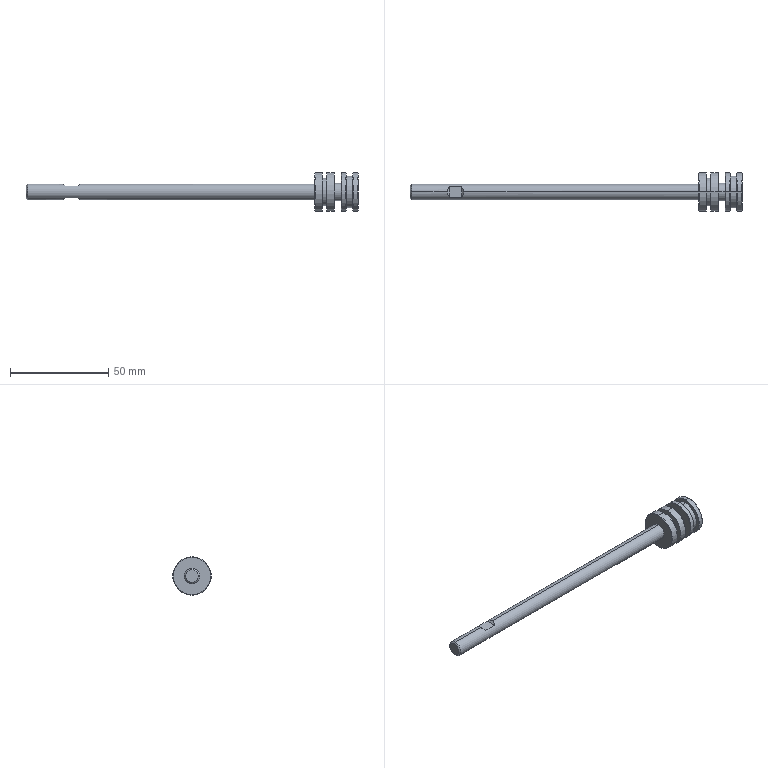Part | STEP file | Copy 2^MA20-80-S-U | 1 solid | 45 faces | box 169 x 19.5 x 19.5 mm | volume 12396 mm3 | cylinder 16 | plane 15 | cone 14 | commonest cylinder face diameters 19.5 x8 8 x2 8.9 x2 14 x2 16 x2
STEP:
#1=CARTESIAN_POINT('',(-55.233,0.,-4.));
#2=VERTEX_POINT('',#1);
#3=CARTESIAN_POINT('',(-55.233,0.,4.));
#4=VERTEX_POINT('',#3);
#5=CARTESIAN_POINT('',(-55.233,0.,0.));
#6=DIRECTION('',(1.,0.,0.));
#7=DIRECTION('',(0.,0.,-1.));
#8=AXIS2_PLACEMENT_3D('',#5,#6,#7);
#9=CIRCLE('',#8,4.);
#10=EDGE_CURVE('',#2,#4,#9,.T.);
#11=ORIENTED_EDGE('',*,*,#10,.T.);
#12=CARTESIAN_POINT('',(-37.,0.,4.));
#13=VERTEX_POINT('',#12);
#14=CARTESIAN_POINT('',(17.884,0.,4.));
#15=DIRECTION('',(1.,0.,0.));
#16=VECTOR('',#15,1000.);
#17=LINE('',#14,#16);
#18=EDGE_CURVE('',#4,#13,#17,.T.);
#19=ORIENTED_EDGE('',*,*,#18,.T.);
#20=CARTESIAN_POINT('',(-36.,2.646,3.));
#21=VERTEX_POINT('',#20);
#22=CARTESIAN_POINT('',(-37.,0.,4.));
#23=CARTESIAN_POINT('',(-37.,0.9852,4.));
#24=CARTESIAN_POINT('',(-36.652,1.907,3.652));
#25=CARTESIAN_POINT('',(-36.,2.646,3.));
#26=(BOUNDED_CURVE()B_SPLINE_CURVE(3,(#22,#23,#24,#25),.UNSPECIFIED.,.F.,.F.)B_SPLINE_CURVE_WITH_KNOTS((4,4),(3.142,3.864),.UNSPECIFIED.)CURVE()GEOMETRIC_REPRESENTATION_ITEM()RATIONAL_B_SPLINE_CURVE((1.,0.9569,0.9569,1.))REPRESENTATION_ITEM(''));
#27=EDGE_CURVE('',#13,#21,#26,.T.);
#28=ORIENTED_EDGE('',*,*,#27,.T.);
#29=CARTESIAN_POINT('',(-29.6,2.646,3.));
#30=VERTEX_POINT('',#29);
#31=CARTESIAN_POINT('',(17.884,2.646,3.));
#32=DIRECTION('',(1.,0.,0.));
#33=VECTOR('',#32,1000.);
#34=LINE('',#31,#33);
#35=EDGE_CURVE('',#21,#30,#34,.T.);
#36=ORIENTED_EDGE('',*,*,#35,.T.);
#37=CARTESIAN_POINT('',(-28.6,0.,4.));
#38=VERTEX_POINT('',#37);
#39=CARTESIAN_POINT('',(-29.6,2.646,3.));
#40=CARTESIAN_POINT('',(-28.948,1.907,3.652));
#41=CARTESIAN_POINT('',(-28.6,0.9852,4.));
#42=CARTESIAN_POINT('',(-28.6,0.,4.));
#43=(BOUNDED_CURVE()B_SPLINE_CURVE(3,(#39,#40,#41,#42),.UNSPECIFIED.,.F.,.F.)B_SPLINE_CURVE_WITH_KNOTS((4,4),(5.56,6.283),.UNSPECIFIED.)CURVE()GEOMETRIC_REPRESENTATION_ITEM()RATIONAL_B_SPLINE_CURVE((1.,0.9569,0.9569,1.))REPRESENTATION_ITEM(''));
#44=EDGE_CURVE('',#30,#38,#43,.T.);
#45=ORIENTED_EDGE('',*,*,#44,.T.);
#46=CARTESIAN_POINT('',(91.,0.,4.));
#47=VERTEX_POINT('',#46);
#48=CARTESIAN_POINT('',(17.884,0.,4.));
#49=DIRECTION('',(1.,0.,0.));
#50=VECTOR('',#49,1000.);
#51=LINE('',#48,#50);
#52=EDGE_CURVE('',#38,#47,#51,.T.);
#53=ORIENTED_EDGE('',*,*,#52,.T.);
#54=CARTESIAN_POINT('',(91.,0.,-4.));
#55=VERTEX_POINT('',#54);
#56=CARTESIAN_POINT('',(91.,0.,0.));
#57=DIRECTION('',(-1.,0.,0.));
#58=DIRECTION('',(0.,0.,-1.));
#59=AXIS2_PLACEMENT_3D('',#56,#57,#58);
#60=CIRCLE('',#59,4.);
#61=EDGE_CURVE('',#47,#55,#60,.T.);
#62=ORIENTED_EDGE('',*,*,#61,.T.);
#63=CARTESIAN_POINT('',(-28.6,0.,-4.));
#64=VERTEX_POINT('',#63);
#65=CARTESIAN_POINT('',(17.884,0.,-4.));
#66=DIRECTION('',(1.,0.,0.));
#67=VECTOR('',#66,1000.);
#68=LINE('',#65,#67);
#69=EDGE_CURVE('',#64,#55,#68,.T.);
#70=ORIENTED_EDGE('',*,*,#69,.F.);
#71=CARTESIAN_POINT('',(-29.6,2.646,-3.));
#72=VERTEX_POINT('',#71);
#73=CARTESIAN_POINT('',(-28.6,0.,-4.));
#74=CARTESIAN_POINT('',(-28.6,0.9852,-4.));
#75=CARTESIAN_POINT('',(-28.948,1.907,-3.652));
#76=CARTESIAN_POINT('',(-29.6,2.646,-3.));
#77=(BOUNDED_CURVE()B_SPLINE_CURVE(3,(#73,#74,#75,#76),.UNSPECIFIED.,.F.,.F.)B_SPLINE_CURVE_WITH_KNOTS((4,4),(0.,0.7227),.UNSPECIFIED.)CURVE()GEOMETRIC_REPRESENTATION_ITEM()RATIONAL_B_SPLINE_CURVE((1.,0.9569,0.9569,1.))REPRESENTATION_ITEM(''));
#78=EDGE_CURVE('',#64,#72,#77,.T.);
#79=ORIENTED_EDGE('',*,*,#78,.T.);
#80=CARTESIAN_POINT('',(-36.,2.646,-3.));
#81=VERTEX_POINT('',#80);
#82=CARTESIAN_POINT('',(17.884,2.646,-3.));
#83=DIRECTION('',(-1.,0.,0.));
#84=VECTOR('',#83,1000.);
#85=LINE('',#82,#84);
#86=EDGE_CURVE('',#72,#81,#85,.T.);
#87=ORIENTED_EDGE('',*,*,#86,.T.);
#88=CARTESIAN_POINT('',(-37.,0.,-4.));
#89=VERTEX_POINT('',#88);
#90=CARTESIAN_POINT('',(-36.,2.646,-3.));
#91=CARTESIAN_POINT('',(-36.652,1.907,-3.652));
#92=CARTESIAN_POINT('',(-37.,0.9852,-4.));
#93=CARTESIAN_POINT('',(-37.,0.,-4.));
#94=(BOUNDED_CURVE()B_SPLINE_CURVE(3,(#90,#91,#92,#93),.UNSPECIFIED.,.F.,.F.)B_SPLINE_CURVE_WITH_KNOTS((4,4),(2.419,3.142),.UNSPECIFIED.)CURVE()GEOMETRIC_REPRESENTATION_ITEM()RATIONAL_B_SPLINE_CURVE((1.,0.9569,0.9569,1.))REPRESENTATION_ITEM(''));
#95=EDGE_CURVE('',#81,#89,#94,.T.);
#96=ORIENTED_EDGE('',*,*,#95,.T.);
#97=CARTESIAN_POINT('',(17.884,0.,-4.));
#98=DIRECTION('',(1.,0.,0.));
#99=VECTOR('',#98,1000.);
#100=LINE('',#97,#99);
#101=EDGE_CURVE('',#2,#89,#100,.T.);
#102=ORIENTED_EDGE('',*,*,#101,.F.);
#103=EDGE_LOOP('',(#11,#19,#28,#36,#45,#53,#62,#70,#79,#87,#96,#102));
#104=FACE_OUTER_BOUND('',#103,.T.);
#105=CARTESIAN_POINT('',(17.884,0.,0.));
#106=DIRECTION('',(1.,0.,0.));
#107=DIRECTION('',(0.,0.,-1.));
#108=AXIS2_PLACEMENT_3D('',#105,#106,#107);
#109=CYLINDRICAL_SURFACE('',#108,4.);
#110=ADVANCED_FACE('',(#104),#109,.T.);
#111=CARTESIAN_POINT('',(-56.,0.,-3.233));
#112=VERTEX_POINT('',#111);
#113=CARTESIAN_POINT('',(-56.,0.,3.233));
#114=VERTEX_POINT('',#113);
#115=CARTESIAN_POINT('',(-56.,0.,0.));
#116=DIRECTION('',(1.,0.,0.));
#117=DIRECTION('',(0.,0.,-1.));
#118=AXIS2_PLACEMENT_3D('',#115,#116,#117);
#119=CIRCLE('',#118,3.233);
#120=EDGE_CURVE('',#112,#114,#119,.T.);
#121=ORIENTED_EDGE('',*,*,#120,.T.);
#122=CARTESIAN_POINT('',(-55.233,0.,4.));
#123=DIRECTION('',(0.7071,0.,0.7071));
#124=VECTOR('',#123,1000.);
#125=LINE('',#122,#124);
#126=EDGE_CURVE('',#114,#4,#125,.T.);
#127=ORIENTED_EDGE('',*,*,#126,.T.);
#128=ORIENTED_EDGE('',*,*,#10,.F.);
#129=CARTESIAN_POINT('',(-55.233,0.,-4.));
#130=DIRECTION('',(0.7071,0.,-0.7071));
#131=VECTOR('',#130,1000.);
#132=LINE('',#129,#131);
#133=EDGE_CURVE('',#112,#2,#132,.T.);
#134=ORIENTED_EDGE('',*,*,#133,.F.);
#135=EDGE_LOOP('',(#121,#127,#128,#134));
#136=FACE_OUTER_BOUND('',#135,.T.);
#137=CARTESIAN_POINT('',(-55.233,0.,0.));
#138=DIRECTION('',(1.,0.,0.));
#139=DIRECTION('',(0.,0.,-1.));
#140=AXIS2_PLACEMENT_3D('',#137,#138,#139);
#141=CONICAL_SURFACE('',#140,4.,0.7854);
#142=ADVANCED_FACE('',(#136),#141,.T.);
#143=CARTESIAN_POINT('',(91.,0.,9.55));
#144=VERTEX_POINT('',#143);
#145=CARTESIAN_POINT('',(91.,0.,-9.55));
#146=VERTEX_POINT('',#145);
#147=CARTESIAN_POINT('',(91.,0.,0.));
#148=DIRECTION('',(-1.,0.,0.));
#149=DIRECTION('',(0.,0.,-1.));
#150=AXIS2_PLACEMENT_3D('',#147,#148,#149);
#151=CIRCLE('',#150,9.55);
#152=EDGE_CURVE('',#144,#146,#151,.T.);
#153=ORIENTED_EDGE('',*,*,#152,.F.);
#154=CARTESIAN_POINT('',(91.2,0.,9.75));
#155=VERTEX_POINT('',#154);
#156=CARTESIAN_POINT('',(91.2,0.,9.75));
#157=DIRECTION('',(0.7071,0.,0.7071));
#158=VECTOR('',#157,1000.);
#159=LINE('',#156,#158);
#160=EDGE_CURVE('',#144,#155,#159,.T.);
#161=ORIENTED_EDGE('',*,*,#160,.T.);
#162=CARTESIAN_POINT('',(91.2,0.,-9.75));
#163=VERTEX_POINT('',#162);
#164=CARTESIAN_POINT('',(91.2,0.,0.));
#165=DIRECTION('',(-1.,0.,0.));
#166=DIRECTION('',(0.,1.,0.));
#167=AXIS2_PLACEMENT_3D('',#164,#165,#166);
#168=CIRCLE('',#167,9.75);
#169=EDGE_CURVE('',#155,#163,#168,.T.);
#170=ORIENTED_EDGE('',*,*,#169,.T.);
#171=CARTESIAN_POINT('',(91.2,0.,-9.75));
#172=DIRECTION('',(0.7071,0.,-0.7071));
#173=VECTOR('',#172,1000.);
#174=LINE('',#171,#173);
#175=EDGE_CURVE('',#146,#163,#174,.T.);
#176=ORIENTED_EDGE('',*,*,#175,.F.);
#177=EDGE_LOOP('',(#153,#161,#170,#176));
#178=FACE_OUTER_BOUND('',#177,.T.);
#179=CARTESIAN_POINT('',(91.2,0.,0.));
#180=DIRECTION('',(1.,0.,0.));
#181=DIRECTION('',(0.,0.,-1.));
#182=AXIS2_PLACEMENT_3D('',#179,#180,#181);
#183=CONICAL_SURFACE('',#182,9.75,0.7854);
#184=ADVANCED_FACE('',(#178),#183,.T.);
#185=ORIENTED_EDGE('',*,*,#169,.F.);
#186=CARTESIAN_POINT('',(94.8,0.,9.75));
#187=VERTEX_POINT('',#186);
#188=CARTESIAN_POINT('',(93.,0.,9.75));
#189=DIRECTION('',(1.,0.,0.));
#190=VECTOR('',#189,1000.);
#191=LINE('',#188,#190);
#192=EDGE_CURVE('',#155,#187,#191,.T.);
#193=ORIENTED_EDGE('',*,*,#192,.T.);
#194=CARTESIAN_POINT('',(94.8,0.,-9.75));
#195=VERTEX_POINT('',#194);
#196=CARTESIAN_POINT('',(94.8,0.,0.));
#197=DIRECTION('',(-1.,0.,0.));
#198=DIRECTION('',(0.,0.,-1.));
#199=AXIS2_PLACEMENT_3D('',#196,#197,#198);
#200=CIRCLE('',#199,9.75);
#201=EDGE_CURVE('',#187,#195,#200,.T.);
#202=ORIENTED_EDGE('',*,*,#201,.T.);
#203=CARTESIAN_POINT('',(93.,0.,-9.75));
#204=DIRECTION('',(1.,0.,0.));
#205=VECTOR('',#204,1000.);
#206=LINE('',#203,#205);
#207=EDGE_CURVE('',#163,#195,#206,.T.);
#208=ORIENTED_EDGE('',*,*,#207,.F.);
#209=EDGE_LOOP('',(#185,#193,#202,#208));
#210=FACE_OUTER_BOUND('',#209,.T.);
#211=CARTESIAN_POINT('',(93.,0.,0.));
#212=DIRECTION('',(1.,0.,0.));
#213=DIRECTION('',(0.,0.,-1.));
#214=AXIS2_PLACEMENT_3D('',#211,#212,#213);
#215=CYLINDRICAL_SURFACE('',#214,9.75);
#216=ADVANCED_FACE('',(#210),#215,.T.);
#217=CARTESIAN_POINT('',(94.8,0.,7.));
#218=VERTEX_POINT('',#217);
#219=CARTESIAN_POINT('',(94.8,0.,-7.));
#220=VERTEX_POINT('',#219);
#221=CARTESIAN_POINT('',(94.8,0.,0.));
#222=DIRECTION('',(-1.,0.,0.));
#223=DIRECTION('',(0.,0.,-1.));
#224=AXIS2_PLACEMENT_3D('',#221,#222,#223);
#225=CIRCLE('',#224,7.);
#226=EDGE_CURVE('',#218,#220,#225,.T.);
#227=ORIENTED_EDGE('',*,*,#226,.F.);
#228=CARTESIAN_POINT('',(97.2,0.,7.));
#229=VERTEX_POINT('',#228);
#230=CARTESIAN_POINT('',(96.,0.,7.));
#231=DIRECTION('',(1.,0.,0.));
#232=VECTOR('',#231,1000.);
#233=LINE('',#230,#232);
#234=EDGE_CURVE('',#218,#229,#233,.T.);
#235=ORIENTED_EDGE('',*,*,#234,.T.);
#236=CARTESIAN_POINT('',(97.2,0.,-7.));
#237=VERTEX_POINT('',#236);
#238=CARTESIAN_POINT('',(97.2,0.,0.));
#239=DIRECTION('',(-1.,0.,0.));
#240=DIRECTION('',(0.,0.,-1.));
#241=AXIS2_PLACEMENT_3D('',#238,#239,#240);
#242=CIRCLE('',#241,7.);
#243=EDGE_CURVE('',#229,#237,#242,.T.);
#244=ORIENTED_EDGE('',*,*,#243,.T.);
#245=CARTESIAN_POINT('',(96.,0.,-7.));
#246=DIRECTION('',(1.,0.,0.));
#247=VECTOR('',#246,1000.);
#248=LINE('',#245,#247);
#249=EDGE_CURVE('',#220,#237,#248,.T.);
#250=ORIENTED_EDGE('',*,*,#249,.F.);
#251=EDGE_LOOP('',(#227,#235,#244,#250));
#252=FACE_OUTER_BOUND('',#251,.T.);
#253=CARTESIAN_POINT('',(96.,0.,0.));
#254=DIRECTION('',(1.,0.,0.));
#255=DIRECTION('',(0.,0.,-1.));
#256=AXIS2_PLACEMENT_3D('',#253,#254,#255);
#257=CYLINDRICAL_SURFACE('',#256,7.);
#258=ADVANCED_FACE('',(#252),#257,.T.);
#259=CARTESIAN_POINT('',(97.2,0.,9.75));
#260=VERTEX_POINT('',#259);
#261=CARTESIAN_POINT('',(97.2,0.,-9.75));
#262=VERTEX_POINT('',#261);
#263=CARTESIAN_POINT('',(97.2,0.,0.));
#264=DIRECTION('',(-1.,0.,0.));
#265=DIRECTION('',(0.,0.,-1.));
#266=AXIS2_PLACEMENT_3D('',#263,#264,#265);
#267=CIRCLE('',#266,9.75);
#268=EDGE_CURVE('',#260,#262,#267,.T.);
#269=ORIENTED_EDGE('',*,*,#268,.F.);
#270=CARTESIAN_POINT('',(100.8,0.,9.75));
#271=VERTEX_POINT('',#270);
#272=CARTESIAN_POINT('',(99.,0.,9.75));
#273=DIRECTION('',(1.,0.,0.));
#274=VECTOR('',#273,1000.);
#275=LINE('',#272,#274);
#276=EDGE_CURVE('',#260,#271,#275,.T.);
#277=ORIENTED_EDGE('',*,*,#276,.T.);
#278=CARTESIAN_POINT('',(100.8,0.,-9.75));
#279=VERTEX_POINT('',#278);
#280=CARTESIAN_POINT('',(100.8,0.,0.));
#281=DIRECTION('',(-1.,0.,0.));
#282=DIRECTION('',(0.,0.,-1.));
#283=AXIS2_PLACEMENT_3D('',#280,#281,#282);
#284=CIRCLE('',#283,9.75);
#285=EDGE_CURVE('',#271,#279,#284,.T.);
#286=ORIENTED_EDGE('',*,*,#285,.T.);
#287=CARTESIAN_POINT('',(99.,0.,-9.75));
#288=DIRECTION('',(1.,0.,0.));
#289=VECTOR('',#288,1000.);
#290=LINE('',#287,#289);
#291=EDGE_CURVE('',#262,#279,#290,.T.);
#292=ORIENTED_EDGE('',*,*,#291,.F.);
#293=EDGE_LOOP('',(#269,#277,#286,#292));
#294=FACE_OUTER_BOUND('',#293,.T.);
#295=CARTESIAN_POINT('',(99.,0.,0.));
#296=DIRECTION('',(1.,0.,0.));
#297=DIRECTION('',(0.,0.,-1.));
#298=AXIS2_PLACEMENT_3D('',#295,#296,#297);
#299=CYLINDRICAL_SURFACE('',#298,9.75);
#300=ADVANCED_FACE('',(#294),#299,.T.);
#301=CARTESIAN_POINT('',(101.,0.,9.55));
#302=VERTEX_POINT('',#301);
#303=CARTESIAN_POINT('',(101.,0.,-9.55));
#304=VERTEX_POINT('',#303);
#305=CARTESIAN_POINT('',(101.,0.,0.));
#306=DIRECTION('',(-1.,0.,0.));
#307=DIRECTION('',(0.,0.,1.));
#308=AXIS2_PLACEMENT_3D('',#305,#306,#307);
#309=CIRCLE('',#308,9.55);
#310=EDGE_CURVE('',#302,#304,#309,.T.);
#311=ORIENTED_EDGE('',*,*,#310,.T.);
#312=CARTESIAN_POINT('',(100.8,0.,-9.75));
#313=DIRECTION('',(-0.7071,0.,-0.7071));
#314=VECTOR('',#313,1000.);
#315=LINE('',#312,#314);
#316=EDGE_CURVE('',#304,#279,#315,.T.);
#317=ORIENTED_EDGE('',*,*,#316,.T.);
#318=ORIENTED_EDGE('',*,*,#285,.F.);
#319=CARTESIAN_POINT('',(100.8,0.,9.75));
#320=DIRECTION('',(-0.7071,0.,0.7071));
#321=VECTOR('',#320,1000.);
#322=LINE('',#319,#321);
#323=EDGE_CURVE('',#302,#271,#322,.T.);
#324=ORIENTED_EDGE('',*,*,#323,.F.);
#325=EDGE_LOOP('',(#311,#317,#318,#324));
#326=FACE_OUTER_BOUND('',#325,.T.);
#327=CARTESIAN_POINT('',(100.8,0.,0.));
#328=DIRECTION('',(-1.,0.,0.));
#329=DIRECTION('',(0.,0.,1.));
#330=AXIS2_PLACEMENT_3D('',#327,#328,#329);
#331=CONICAL_SURFACE('',#330,9.75,0.7854);
#332=ADVANCED_FACE('',(#326),#331,.T.);
#333=CARTESIAN_POINT('',(101.,0.,4.45));
#334=VERTEX_POINT('',#333);
#335=CARTESIAN_POINT('',(101.,0.,-4.45));
#336=VERTEX_POINT('',#335);
#337=CARTESIAN_POINT('',(101.,0.,0.));
#338=DIRECTION('',(-1.,0.,0.));
#339=DIRECTION('',(0.,0.,-1.));
#340=AXIS2_PLACEMENT_3D('',#337,#338,#339);
#341=CIRCLE('',#340,4.45);
#342=EDGE_CURVE('',#334,#336,#341,.T.);
#343=ORIENTED_EDGE('',*,*,#342,.F.);
#344=CARTESIAN_POINT('',(104.5,0.,4.45));
#345=VERTEX_POINT('',#344);
#346=CARTESIAN_POINT('',(102.75,0.,4.45));
#347=DIRECTION('',(1.,0.,0.));
#348=VECTOR('',#347,1000.);
#349=LINE('',#346,#348);
#350=EDGE_CURVE('',#334,#345,#349,.T.);
#351=ORIENTED_EDGE('',*,*,#350,.T.);
#352=CARTESIAN_POINT('',(104.5,0.,-4.45));
#353=VERTEX_POINT('',#352);
#354=CARTESIAN_POINT('',(104.5,0.,0.));
#355=DIRECTION('',(-1.,0.,0.));
#356=DIRECTION('',(0.,0.,-1.));
#357=AXIS2_PLACEMENT_3D('',#354,#355,#356);
#358=CIRCLE('',#357,4.45);
#359=EDGE_CURVE('',#345,#353,#358,.T.);
#360=ORIENTED_EDGE('',*,*,#359,.T.);
#361=CARTESIAN_POINT('',(102.75,0.,-4.45));
#362=DIRECTION('',(1.,0.,0.));
#363=VECTOR('',#362,1000.);
#364=LINE('',#361,#363);
#365=EDGE_CURVE('',#336,#353,#364,.T.);
#366=ORIENTED_EDGE('',*,*,#365,.F.);
#367=EDGE_LOOP('',(#343,#351,#360,#366));
#368=FACE_OUTER_BOUND('',#367,.T.);
#369=CARTESIAN_POINT('',(102.75,0.,0.));
#370=DIRECTION('',(1.,0.,0.));
#371=DIRECTION('',(0.,0.,-1.));
#372=AXIS2_PLACEMENT_3D('',#369,#370,#371);
#373=CYLINDRICAL_SURFACE('',#372,4.45);
#374=ADVANCED_FACE('',(#368),#373,.T.);
#375=CARTESIAN_POINT('',(104.5,0.,9.55));
#376=VERTEX_POINT('',#375);
#377=CARTESIAN_POINT('',(104.5,0.,-9.55));
#378=VERTEX_POINT('',#377);
#379=CARTESIAN_POINT('',(104.5,0.,0.));
#380=DIRECTION('',(-1.,0.,0.));
#381=DIRECTION('',(0.,0.,-1.));
#382=AXIS2_PLACEMENT_3D('',#379,#380,#381);
#383=CIRCLE('',#382,9.55);
#384=EDGE_CURVE('',#376,#378,#383,.T.);
#385=ORIENTED_EDGE('',*,*,#384,.F.);
#386=CARTESIAN_POINT('',(104.7,0.,9.75));
#387=VERTEX_POINT('',#386);
#388=CARTESIAN_POINT('',(104.7,0.,9.75));
#389=DIRECTION('',(0.7071,0.,0.7071));
#390=VECTOR('',#389,1000.);
#391=LINE('',#388,#390);
#392=EDGE_CURVE('',#376,#387,#391,.T.);
#393=ORIENTED_EDGE('',*,*,#392,.T.);
#394=CARTESIAN_POINT('',(104.7,0.,-9.75));
#395=VERTEX_POINT('',#394);
#396=CARTESIAN_POINT('',(104.7,0.,0.));
#397=DIRECTION('',(-1.,0.,0.));
#398=DIRECTION('',(0.,1.,0.));
#399=AXIS2_PLACEMENT_3D('',#396,#397,#398);
#400=CIRCLE('',#399,9.75);
#401=EDGE_CURVE('',#387,#395,#400,.T.);
#402=ORIENTED_EDGE('',*,*,#401,.T.);
#403=CARTESIAN_POINT('',(104.7,0.,-9.75));
#404=DIRECTION('',(0.7071,0.,-0.7071));
#405=VECTOR('',#404,1000.);
#406=LINE('',#403,#405);
#407=EDGE_CURVE('',#378,#395,#406,.T.);
#408=ORIENTED_EDGE('',*,*,#407,.F.);
#409=EDGE_LOOP('',(#385,#393,#402,#408));
#410=FACE_OUTER_BOUND('',#409,.T.);
#411=CARTESIAN_POINT('',(104.7,0.,0.));
#412=DIRECTION('',(1.,0.,0.));
#413=DIRECTION('',(0.,0.,-1.));
#414=AXIS2_PLACEMENT_3D('',#411,#412,#413);
#415=CONICAL_SURFACE('',#414,9.75,0.7854);
#416=ADVANCED_FACE('',(#410),#415,.T.);
#417=ORIENTED_EDGE('',*,*,#401,.F.);
#418=CARTESIAN_POINT('',(106.85,0.,9.75));
#419=VERTEX_POINT('',#418);
#420=CARTESIAN_POINT('',(105.775,0.,9.75));
#421=DIRECTION('',(1.,0.,0.));
#422=VECTOR('',#421,1000.);
#423=LINE('',#420,#422);
#424=EDGE_CURVE('',#387,#419,#423,.T.);
#425=ORIENTED_EDGE('',*,*,#424,.T.);
#426=CARTESIAN_POINT('',(106.85,0.,-9.75));
#427=VERTEX_POINT('',#426);
#428=CARTESIAN_POINT('',(106.85,0.,0.));
#429=DIRECTION('',(-1.,0.,0.));
#430=DIRECTION('',(0.,0.,-1.));
#431=AXIS2_PLACEMENT_3D('',#428,#429,#430);
#432=CIRCLE('',#431,9.75);
#433=EDGE_CURVE('',#419,#427,#432,.T.);
#434=ORIENTED_EDGE('',*,*,#433,.T.);
#435=CARTESIAN_POINT('',(105.775,0.,-9.75));
#436=DIRECTION('',(1.,0.,0.));
#437=VECTOR('',#436,1000.);
#438=LINE('',#435,#437);
#439=EDGE_CURVE('',#395,#427,#438,.T.);
#440=ORIENTED_EDGE('',*,*,#439,.F.);
#441=EDGE_LOOP('',(#417,#425,#434,#440));
#442=FACE_OUTER_BOUND('',#441,.T.);
#443=CARTESIAN_POINT('',(105.775,0.,0.));
#444=DIRECTION('',(1.,0.,0.));
#445=DIRECTION('',(0.,0.,-1.));
#446=AXIS2_PLACEMENT_3D('',#443,#444,#445);
#447=CYLINDRICAL_SURFACE('',#446,9.75);
#448=ADVANCED_FACE('',(#442),#447,.T.);
#449=CARTESIAN_POINT('',(107.05,0.,9.55));
#450=VERTEX_POINT('',#449);
#451=CARTESIAN_POINT('',(107.05,0.,-9.55));
#452=VERTEX_POINT('',#451);
#453=CARTESIAN_POINT('',(107.05,0.,0.));
#454=DIRECTION('',(-1.,0.,0.));
#455=DIRECTION('',(0.,0.,1.));
#456=AXIS2_PLACEMENT_3D('',#453,#454,#455);
#457=CIRCLE('',#456,9.55);
#458=EDGE_CURVE('',#450,#452,#457,.T.);
#459=ORIENTED_EDGE('',*,*,#458,.T.);
#460=CARTESIAN_POINT('',(106.85,0.,-9.75));
#461=DIRECTION('',(-0.7071,0.,-0.7071));
#462=VECTOR('',#461,1000.);
#463=LINE('',#460,#462);
#464=EDGE_CURVE('',#452,#427,#463,.T.);
#465=ORIENTED_EDGE('',*,*,#464,.T.);
#466=ORIENTED_EDGE('',*,*,#433,.F.);
#467=CARTESIAN_POINT('',(106.85,0.,9.75));
#468=DIRECTION('',(-0.7071,0.,0.7071));
#469=VECTOR('',#468,1000.);
#470=LINE('',#467,#469);
#471=EDGE_CURVE('',#450,#419,#470,.T.);
#472=ORIENTED_EDGE('',*,*,#471,.F.);
#473=EDGE_LOOP('',(#459,#465,#466,#472));
#474=FACE_OUTER_BOUND('',#473,.T.);
#475=CARTESIAN_POINT('',(106.85,0.,0.));
#476=DIRECTION('',(-1.,0.,0.));
#477=DIRECTION('',(0.,0.,1.));
#478=AXIS2_PLACEMENT_3D('',#475,#476,#477);
#479=CONICAL_SURFACE('',#478,9.75,0.7854);
#480=ADVANCED_FACE('',(#474),#479,.T.);
#481=CARTESIAN_POINT('',(107.05,0.,8.));
#482=VERTEX_POINT('',#481);
#483=CARTESIAN_POINT('',(107.05,0.,-8.));
#484=VERTEX_POINT('',#483);
#485=CARTESIAN_POINT('',(107.05,0.,0.));
#486=DIRECTION('',(-1.,0.,0.));
#487=DIRECTION('',(0.,0.,-1.));
#488=AXIS2_PLACEMENT_3D('',#485,#486,#487);
#489=CIRCLE('',#488,8.);
#490=EDGE_CURVE('',#482,#484,#489,.T.);
#491=ORIENTED_EDGE('',*,*,#490,.F.);
#492=CARTESIAN_POINT('',(110.35,0.,8.));
#493=VERTEX_POINT('',#492);
#494=CARTESIAN_POINT('',(108.7,0.,8.));
#495=DIRECTION('',(1.,0.,0.));
#496=VECTOR('',#495,1000.);
#497=LINE('',#494,#496);
#498=EDGE_CURVE('',#482,#493,#497,.T.);
#499=ORIENTED_EDGE('',*,*,#498,.T.);
#500=CARTESIAN_POINT('',(110.35,0.,-8.));
#501=VERTEX_POINT('',#500);
#502=CARTESIAN_POINT('',(110.35,0.,0.));
#503=DIRECTION('',(-1.,0.,0.));
#504=DIRECTION('',(0.,0.,-1.));
#505=AXIS2_PLACEMENT_3D('',#502,#503,#504);
#506=CIRCLE('',#505,8.);
#507=EDGE_CURVE('',#493,#501,#506,.T.);
#508=ORIENTED_EDGE('',*,*,#507,.T.);
#509=CARTESIAN_POINT('',(108.7,0.,-8.));
#510=DIRECTION('',(1.,0.,0.));
#511=VECTOR('',#510,1000.);
#512=LINE('',#509,#511);
#513=EDGE_CURVE('',#484,#501,#512,.T.);
#514=ORIENTED_EDGE('',*,*,#513,.F.);
#515=EDGE_LOOP('',(#491,#499,#508,#514));
#516=FACE_OUTER_BOUND('',#515,.T.);
#517=CARTESIAN_POINT('',(108.7,0.,0.));
#518=DIRECTION('',(1.,0.,0.));
#519=DIRECTION('',(0.,0.,-1.));
#520=AXIS2_PLACEMENT_3D('',#517,#518,#519);
#521=CYLINDRICAL_SURFACE('',#520,8.);
#522=ADVANCED_FACE('',(#516),#521,.T.);
#523=CARTESIAN_POINT('',(110.35,0.,9.55));
#524=VERTEX_POINT('',#523);
#525=CARTESIAN_POINT('',(110.35,0.,-9.55));
#526=VERTEX_POINT('',#525);
#527=CARTESIAN_POINT('',(110.35,0.,0.));
#528=DIRECTION('',(-1.,0.,0.));
#529=DIRECTION('',(0.,0.,-1.));
#530=AXIS2_PLACEMENT_3D('',#527,#528,#529);
#531=CIRCLE('',#530,9.55);
#532=EDGE_CURVE('',#524,#526,#531,.T.);
#533=ORIENTED_EDGE('',*,*,#532,.F.);
#534=CARTESIAN_POINT('',(110.55,0.,9.75));
#535=VERTEX_POINT('',#534);
#536=CARTESIAN_POINT('',(110.55,0.,9.75));
#537=DIRECTION('',(0.7071,0.,0.7071));
#538=VECTOR('',#537,1000.);
#539=LINE('',#536,#538);
#540=EDGE_CURVE('',#524,#535,#539,.T.);
#541=ORIENTED_EDGE('',*,*,#540,.T.);
#542=CARTESIAN_POINT('',(110.55,0.,-9.75));
#543=VERTEX_POINT('',#542);
#544=CARTESIAN_POINT('',(110.55,0.,0.));
#545=DIRECTION('',(-1.,0.,0.));
#546=DIRECTION('',(0.,1.,0.));
#547=AXIS2_PLACEMENT_3D('',#544,#545,#546);
#548=CIRCLE('',#547,9.75);
#549=EDGE_CURVE('',#535,#543,#548,.T.);
#550=ORIENTED_EDGE('',*,*,#549,.T.);
#551=CARTESIAN_POINT('',(110.55,0.,-9.75));
#552=DIRECTION('',(0.7071,0.,-0.7071));
#553=VECTOR('',#552,1000.);
#554=LINE('',#551,#553);
#555=EDGE_CURVE('',#526,#543,#554,.T.);
#556=ORIENTED_EDGE('',*,*,#555,.F.);
#557=EDGE_LOOP('',(#533,#541,#550,#556));
#558=FACE_OUTER_BOUND('',#557,.T.);
#559=CARTESIAN_POINT('',(110.55,0.,0.));
#560=DIRECTION('',(1.,0.,0.));
#561=DIRECTION('',(0.,0.,-1.));
#562=AXIS2_PLACEMENT_3D('',#559,#560,#561);
#563=CONICAL_SURFACE('',#562,9.75,0.7854);
#564=ADVANCED_FACE('',(#558),#563,.T.);
#565=ORIENTED_EDGE('',*,*,#549,.F.);
#566=CARTESIAN_POINT('',(112.8,0.,9.75));
#567=VERTEX_POINT('',#566);
#568=CARTESIAN_POINT('',(111.675,0.,9.75));
#569=DIRECTION('',(1.,0.,0.));
#570=VECTOR('',#569,1000.);
#571=LINE('',#568,#570);
#572=EDGE_CURVE('',#535,#567,#571,.T.);
#573=ORIENTED_EDGE('',*,*,#572,.T.);
#574=CARTESIAN_POINT('',(112.8,0.,-9.75));
#575=VERTEX_POINT('',#574);
#576=CARTESIAN_POINT('',(112.8,0.,0.));
#577=DIRECTION('',(-1.,0.,0.));
#578=DIRECTION('',(0.,0.,-1.));
#579=AXIS2_PLACEMENT_3D('',#576,#577,#578);
#580=CIRCLE('',#579,9.75);
#581=EDGE_CURVE('',#567,#575,#580,.T.);
#582=ORIENTED_EDGE('',*,*,#581,.T.);
#583=CARTESIAN_POINT('',(111.675,0.,-9.75));
#584=DIRECTION('',(1.,0.,0.));
#585=VECTOR('',#584,1000.);
#586=LINE('',#583,#585);
#587=EDGE_CURVE('',#543,#575,#586,.T.);
#588=ORIENTED_EDGE('',*,*,#587,.F.);
#589=EDGE_LOOP('',(#565,#573,#582,#588));
#590=FACE_OUTER_BOUND('',#589,.T.);
#591=CARTESIAN_POINT('',(111.675,0.,0.));
#592=DIRECTION('',(1.,0.,0.));
#593=DIRECTION('',(0.,0.,-1.));
#594=AXIS2_PLACEMENT_3D('',#591,#592,#593);
#595=CYLINDRICAL_SURFACE('',#594,9.75);
#596=ADVANCED_FACE('',(#590),#595,.T.);
#597=CARTESIAN_POINT('',(113.,0.,9.55));
#598=VERTEX_POINT('',#597);
#599=CARTESIAN_POINT('',(113.,0.,-9.55));
#600=VERTEX_POINT('',#599);
#601=CARTESIAN_POINT('',(113.,0.,0.));
#602=DIRECTION('',(-1.,0.,0.));
#603=DIRECTION('',(0.,0.,1.));
#604=AXIS2_PLACEMENT_3D('',#601,#602,#603);
#605=CIRCLE('',#604,9.55);
#606=EDGE_CURVE('',#598,#600,#605,.T.);
#607=ORIENTED_EDGE('',*,*,#606,.T.);
#608=CARTESIAN_POINT('',(112.8,0.,-9.75));
#609=DIRECTION('',(-0.7071,0.,-0.7071));
#610=VECTOR('',#609,1000.);
#611=LINE('',#608,#610);
#612=EDGE_CURVE('',#600,#575,#611,.T.);
#613=ORIENTED_EDGE('',*,*,#612,.T.);
#614=ORIENTED_EDGE('',*,*,#581,.F.);
#615=CARTESIAN_POINT('',(112.8,0.,9.75));
#616=DIRECTION('',(-0.7071,0.,0.7071));
#617=VECTOR('',#616,1000.);
#618=LINE('',#615,#617);
#619=EDGE_CURVE('',#598,#567,#618,.T.);
#620=ORIENTED_EDGE('',*,*,#619,.F.);
#621=EDGE_LOOP('',(#607,#613,#614,#620));
#622=FACE_OUTER_BOUND('',#621,.T.);
#623=CARTESIAN_POINT('',(112.8,0.,0.));
#624=DIRECTION('',(-1.,0.,0.));
#625=DIRECTION('',(0.,0.,1.));
#626=AXIS2_PLACEMENT_3D('',#623,#624,#625);
#627=CONICAL_SURFACE('',#626,9.75,0.7854);
#628=ADVANCED_FACE('',(#622),#627,.T.);
#629=ORIENTED_EDGE('',*,*,#18,.F.);
#630=CARTESIAN_POINT('',(-55.233,0.,0.));
#631=DIRECTION('',(1.,0.,0.));
#632=DIRECTION('',(0.,0.,-1.));
#633=AXIS2_PLACEMENT_3D('',#630,#631,#632);
#634=CIRCLE('',#633,4.);
#635=EDGE_CURVE('',#4,#2,#634,.T.);
#636=ORIENTED_EDGE('',*,*,#635,.T.);
#637=ORIENTED_EDGE('',*,*,#101,.T.);
#638=CARTESIAN_POINT('',(-36.,-2.646,-3.));
#639=VERTEX_POINT('',#638);
#640=CARTESIAN_POINT('',(-37.,0.,-4.));
#641=CARTESIAN_POINT('',(-37.,-0.9852,-4.));
#642=CARTESIAN_POINT('',(-36.652,-1.907,-3.652));
#643=CARTESIAN_POINT('',(-36.,-2.646,-3.));
#644=(BOUNDED_CURVE()B_SPLINE_CURVE(3,(#640,#641,#642,#643),.UNSPECIFIED.,.F.,.F.)B_SPLINE_CURVE_WITH_KNOTS((4,4),(3.142,3.864),.UNSPECIFIED.)CURVE()GEOMETRIC_REPRESENTATION_ITEM()RATIONAL_B_SPLINE_CURVE((1.,0.9569,0.9569,1.))REPRESENTATION_ITEM(''));
#645=EDGE_CURVE('',#89,#639,#644,.T.);
#646=ORIENTED_EDGE('',*,*,#645,.T.);
#647=CARTESIAN_POINT('',(-29.6,-2.646,-3.));
#648=VERTEX_POINT('',#647);
#649=CARTESIAN_POINT('',(17.884,-2.646,-3.));
#650=DIRECTION('',(1.,0.,0.));
#651=VECTOR('',#650,1000.);
#652=LINE('',#649,#651);
#653=EDGE_CURVE('',#639,#648,#652,.T.);
#654=ORIENTED_EDGE('',*,*,#653,.T.);
#655=CARTESIAN_POINT('',(-29.6,-2.646,-3.));
#656=CARTESIAN_POINT('',(-28.948,-1.907,-3.652));
#657=CARTESIAN_POINT('',(-28.6,-0.9852,-4.));
#658=CARTESIAN_POINT('',(-28.6,0.,-4.));
#659=(BOUNDED_CURVE()B_SPLINE_CURVE(3,(#655,#656,#657,#658),.UNSPECIFIED.,.F.,.F.)B_SPLINE_CURVE_WITH_KNOTS((4,4),(5.56,6.283),.UNSPECIFIED.)CURVE()GEOMETRIC_REPRESENTATION_ITEM()RATIONAL_B_SPLINE_CURVE((1.,0.9569,0.9569,1.))REPRESENTATION_ITEM(''));
#660=EDGE_CURVE('',#648,#64,#659,.T.);
#661=ORIENTED_EDGE('',*,*,#660,.T.);
#662=ORIENTED_EDGE('',*,*,#69,.T.);
#663=CARTESIAN_POINT('',(91.,0.,0.));
#664=DIRECTION('',(-1.,0.,0.));
#665=DIRECTION('',(0.,0.,-1.));
#666=AXIS2_PLACEMENT_3D('',#663,#664,#665);
#667=CIRCLE('',#666,4.);
#668=EDGE_CURVE('',#55,#47,#667,.T.);
#669=ORIENTED_EDGE('',*,*,#668,.T.);
#670=ORIENTED_EDGE('',*,*,#52,.F.);
#671=CARTESIAN_POINT('',(-29.6,-2.646,3.));
#672=VERTEX_POINT('',#671);
#673=CARTESIAN_POINT('',(-28.6,0.,4.));
#674=CARTESIAN_POINT('',(-28.6,-0.9852,4.));
#675=CARTESIAN_POINT('',(-28.948,-1.907,3.652));
#676=CARTESIAN_POINT('',(-29.6,-2.646,3.));
#677=(BOUNDED_CURVE()B_SPLINE_CURVE(3,(#673,#674,#675,#676),.UNSPECIFIED.,.F.,.F.)B_SPLINE_CURVE_WITH_KNOTS((4,4),(0.,0.7227),.UNSPECIFIED.)CURVE()GEOMETRIC_REPRESENTATION_ITEM()RATIONAL_B_SPLINE_CURVE((1.,0.9569,0.9569,1.))REPRESENTATION_ITEM(''));
#678=EDGE_CURVE('',#38,#672,#677,.T.);
#679=ORIENTED_EDGE('',*,*,#678,.T.);
#680=CARTESIAN_POINT('',(-36.,-2.646,3.));
#681=VERTEX_POINT('',#680);
#682=CARTESIAN_POINT('',(17.884,-2.646,3.));
#683=DIRECTION('',(-1.,0.,0.));
#684=VECTOR('',#683,1000.);
#685=LINE('',#682,#684);
#686=EDGE_CURVE('',#672,#681,#685,.T.);
#687=ORIENTED_EDGE('',*,*,#686,.T.);
#688=CARTESIAN_POINT('',(-36.,-2.646,3.));
#689=CARTESIAN_POINT('',(-36.652,-1.907,3.652));
#690=CARTESIAN_POINT('',(-37.,-0.9852,4.));
#691=CARTESIAN_POINT('',(-37.,0.,4.));
#692=(BOUNDED_CURVE()B_SPLINE_CURVE(3,(#688,#689,#690,#691),.UNSPECIFIED.,.F.,.F.)B_SPLINE_CURVE_WITH_KNOTS((4,4),(2.419,3.142),.UNSPECIFIED.)CURVE()GEOMETRIC_REPRESENTATION_ITEM()RATIONAL_B_SPLINE_CURVE((1.,0.9569,0.9569,1.))REPRESENTATION_ITEM(''));
#693=EDGE_CURVE('',#681,#13,#692,.T.);
#694=ORIENTED_EDGE('',*,*,#693,.T.);
#695=EDGE_LOOP('',(#629,#636,#637,#646,#654,#661,#662,#669,#670,#679,#687,#694));
#696=FACE_OUTER_BOUND('',#695,.T.);
#697=CARTESIAN_POINT('',(17.884,0.,0.));
#698=DIRECTION('',(1.,0.,0.));
#699=DIRECTION('',(0.,0.,-1.));
#700=AXIS2_PLACEMENT_3D('',#697,#698,#699);
#701=CYLINDRICAL_SURFACE('',#700,4.);
#702=ADVANCED_FACE('',(#696),#701,.T.);
#703=CARTESIAN_POINT('',(-29.6,3.,3.));
#704=DIRECTION('',(0.,-1.,0.));
#705=VECTOR('',#704,1000.);
#706=LINE('',#703,#705);
#707=EDGE_CURVE('',#30,#672,#706,.T.);
#708=ORIENTED_EDGE('',*,*,#707,.F.);
#709=ORIENTED_EDGE('',*,*,#35,.F.);
#710=CARTESIAN_POINT('',(-36.,3.,3.));
#711=DIRECTION('',(0.,1.,0.));
#712=VECTOR('',#711,1000.);
#713=LINE('',#710,#712);
#714=EDGE_CURVE('',#681,#21,#713,.T.);
#715=ORIENTED_EDGE('',*,*,#714,.F.);
#716=ORIENTED_EDGE('',*,*,#686,.F.);
#717=EDGE_LOOP('',(#708,#709,#715,#716));
#718=FACE_OUTER_BOUND('',#717,.T.);
#719=CARTESIAN_POINT('',(-29.6,3.,3.));
#720=DIRECTION('',(0.,0.,-1.));
#721=DIRECTION('',(-1.,0.,0.));
#722=AXIS2_PLACEMENT_3D('',#719,#720,#721);
#723=PLANE('',#722);
#724=ADVANCED_FACE('',(#718),#723,.F.);
#725=ORIENTED_EDGE('',*,*,#714,.T.);
#726=ORIENTED_EDGE('',*,*,#27,.F.);
#727=ORIENTED_EDGE('',*,*,#693,.F.);
#728=EDGE_LOOP('',(#725,#726,#727));
#729=FACE_OUTER_BOUND('',#728,.T.);
#730=CARTESIAN_POINT('',(-36.,3.,3.));
#731=DIRECTION('',(-0.7071,0.,-0.7071));
#732=DIRECTION('',(-0.7071,0.,0.7071));
#733=AXIS2_PLACEMENT_3D('',#730,#731,#732);
#734=PLANE('',#733);
#735=ADVANCED_FACE('',(#729),#734,.F.);
#736=ORIENTED_EDGE('',*,*,#707,.T.);
#737=ORIENTED_EDGE('',*,*,#678,.F.);
#738=ORIENTED_EDGE('',*,*,#44,.F.);
#739=EDGE_LOOP('',(#736,#737,#738));
#740=FACE_OUTER_BOUND('',#739,.T.);
#741=CARTESIAN_POINT('',(-20.6,3.,12.));
#742=DIRECTION('',(0.7071,0.,-0.7071));
#743=DIRECTION('',(-0.7071,0.,-0.7071));
#744=AXIS2_PLACEMENT_3D('',#741,#742,#743);
#745=PLANE('',#744);
#746=ADVANCED_FACE('',(#740),#745,.F.);
#747=CARTESIAN_POINT('',(91.,0.,0.));
#748=DIRECTION('',(-1.,0.,0.));
#749=DIRECTION('',(0.,0.,-1.));
#750=AXIS2_PLACEMENT_3D('',#747,#748,#749);
#751=CIRCLE('',#750,9.55);
#752=EDGE_CURVE('',#146,#144,#751,.T.);
#753=ORIENTED_EDGE('',*,*,#752,.T.);
#754=ORIENTED_EDGE('',*,*,#152,.T.);
#755=EDGE_LOOP('',(#753,#754));
#756=FACE_OUTER_BOUND('',#755,.T.);
#757=ORIENTED_EDGE('',*,*,#668,.F.);
#758=ORIENTED_EDGE('',*,*,#61,.F.);
#759=EDGE_LOOP('',(#757,#758));
#760=FACE_BOUND('',#759,.T.);
#761=CARTESIAN_POINT('',(91.,6.775,0.));
#762=DIRECTION('',(-1.,0.,0.));
#763=DIRECTION('',(0.,0.,1.));
#764=AXIS2_PLACEMENT_3D('',#761,#762,#763);
#765=PLANE('',#764);
#766=ADVANCED_FACE('',(#756,#760),#765,.T.);
#767=ORIENTED_EDGE('',*,*,#126,.F.);
#768=CARTESIAN_POINT('',(-56.,0.,0.));
#769=DIRECTION('',(1.,0.,0.));
#770=DIRECTION('',(0.,0.,-1.));
#771=AXIS2_PLACEMENT_3D('',#768,#769,#770);
#772=CIRCLE('',#771,3.233);
#773=EDGE_CURVE('',#114,#112,#772,.T.);
#774=ORIENTED_EDGE('',*,*,#773,.T.);
#775=ORIENTED_EDGE('',*,*,#133,.T.);
#776=ORIENTED_EDGE('',*,*,#635,.F.);
#777=EDGE_LOOP('',(#767,#774,#775,#776));
#778=FACE_OUTER_BOUND('',#777,.T.);
#779=CARTESIAN_POINT('',(-55.233,0.,0.));
#780=DIRECTION('',(1.,0.,0.));
#781=DIRECTION('',(0.,0.,-1.));
#782=AXIS2_PLACEMENT_3D('',#779,#780,#781);
#783=CONICAL_SURFACE('',#782,4.,0.7854);
#784=ADVANCED_FACE('',(#778),#783,.T.);
#785=ORIENTED_EDGE('',*,*,#160,.F.);
#786=ORIENTED_EDGE('',*,*,#752,.F.);
#787=ORIENTED_EDGE('',*,*,#175,.T.);
#788=CARTESIAN_POINT('',(91.2,0.,0.));
#789=DIRECTION('',(-1.,0.,0.));
#790=DIRECTION('',(0.,1.,0.));
#791=AXIS2_PLACEMENT_3D('',#788,#789,#790);
#792=CIRCLE('',#791,9.75);
#793=EDGE_CURVE('',#163,#155,#792,.T.);
#794=ORIENTED_EDGE('',*,*,#793,.T.);
#795=EDGE_LOOP('',(#785,#786,#787,#794));
#796=FACE_OUTER_BOUND('',#795,.T.);
#797=CARTESIAN_POINT('',(91.2,0.,0.));
#798=DIRECTION('',(1.,0.,0.));
#799=DIRECTION('',(0.,0.,-1.));
#800=AXIS2_PLACEMENT_3D('',#797,#798,#799);
#801=CONICAL_SURFACE('',#800,9.75,0.7854);
#802=ADVANCED_FACE('',(#796),#801,.T.);
#803=CARTESIAN_POINT('',(-36.,3.,-3.));
#804=DIRECTION('',(0.,-1.,0.));
#805=VECTOR('',#804,1000.);
#806=LINE('',#803,#805);
#807=EDGE_CURVE('',#81,#639,#806,.T.);
#808=ORIENTED_EDGE('',*,*,#807,.F.);
#809=ORIENTED_EDGE('',*,*,#86,.F.);
#810=CARTESIAN_POINT('',(-29.6,3.,-3.));
#811=DIRECTION('',(0.,1.,0.));
#812=VECTOR('',#811,1000.);
#813=LINE('',#810,#812);
#814=EDGE_CURVE('',#648,#72,#813,.T.);
#815=ORIENTED_EDGE('',*,*,#814,.F.);
#816=ORIENTED_EDGE('',*,*,#653,.F.);
#817=EDGE_LOOP('',(#808,#809,#815,#816));
#818=FACE_OUTER_BOUND('',#817,.T.);
#819=CARTESIAN_POINT('',(-36.,3.,-3.));
#820=DIRECTION('',(0.,0.,1.));
#821=DIRECTION('',(1.,0.,0.));
#822=AXIS2_PLACEMENT_3D('',#819,#820,#821);
#823=PLANE('',#822);
#824=ADVANCED_FACE('',(#818),#823,.F.);
#825=ORIENTED_EDGE('',*,*,#814,.T.);
#826=ORIENTED_EDGE('',*,*,#78,.F.);
#827=ORIENTED_EDGE('',*,*,#660,.F.);
#828=EDGE_LOOP('',(#825,#826,#827));
#829=FACE_OUTER_BOUND('',#828,.T.);
#830=CARTESIAN_POINT('',(-29.6,3.,-3.));
#831=DIRECTION('',(0.7071,0.,0.7071));
#832=DIRECTION('',(0.7071,0.,-0.7071));
#833=AXIS2_PLACEMENT_3D('',#830,#831,#832);
#834=PLANE('',#833);
#835=ADVANCED_FACE('',(#829),#834,.F.);
#836=ORIENTED_EDGE('',*,*,#807,.T.);
#837=ORIENTED_EDGE('',*,*,#645,.F.);
#838=ORIENTED_EDGE('',*,*,#95,.F.);
#839=EDGE_LOOP('',(#836,#837,#838));
#840=FACE_OUTER_BOUND('',#839,.T.);
#841=CARTESIAN_POINT('',(-38.,3.,-5.));
#842=DIRECTION('',(-0.7071,0.,0.7071));
#843=DIRECTION('',(0.7071,0.,0.7071));
#844=AXIS2_PLACEMENT_3D('',#841,#842,#843);
#845=PLANE('',#844);
#846=ADVANCED_FACE('',(#840),#845,.F.);
#847=ORIENTED_EDGE('',*,*,#120,.F.);
#848=ORIENTED_EDGE('',*,*,#773,.F.);
#849=EDGE_LOOP('',(#847,#848));
#850=FACE_OUTER_BOUND('',#849,.T.);
#851=CARTESIAN_POINT('',(-56.,1.617,0.));
#852=DIRECTION('',(-1.,0.,0.));
#853=DIRECTION('',(0.,0.,1.));
#854=AXIS2_PLACEMENT_3D('',#851,#852,#853);
#855=PLANE('',#854);
#856=ADVANCED_FACE('',(#850),#855,.T.);
#857=ORIENTED_EDGE('',*,*,#192,.F.);
#858=ORIENTED_EDGE('',*,*,#793,.F.);
#859=ORIENTED_EDGE('',*,*,#207,.T.);
#860=CARTESIAN_POINT('',(94.8,0.,0.));
#861=DIRECTION('',(-1.,0.,0.));
#862=DIRECTION('',(0.,0.,-1.));
#863=AXIS2_PLACEMENT_3D('',#860,#861,#862);
#864=CIRCLE('',#863,9.75);
#865=EDGE_CURVE('',#195,#187,#864,.T.);
#866=ORIENTED_EDGE('',*,*,#865,.T.);
#867=EDGE_LOOP('',(#857,#858,#859,#866));
#868=FACE_OUTER_BOUND('',#867,.T.);
#869=CARTESIAN_POINT('',(93.,0.,0.));
#870=DIRECTION('',(1.,0.,0.));
#871=DIRECTION('',(0.,0.,-1.));
#872=AXIS2_PLACEMENT_3D('',#869,#870,#871);
#873=CYLINDRICAL_SURFACE('',#872,9.75);
#874=ADVANCED_FACE('',(#868),#873,.T.);
#875=CARTESIAN_POINT('',(94.8,0.,0.));
#876=DIRECTION('',(-1.,0.,0.));
#877=DIRECTION('',(0.,0.,-1.));
#878=AXIS2_PLACEMENT_3D('',#875,#876,#877);
#879=CIRCLE('',#878,7.);
#880=EDGE_CURVE('',#220,#218,#879,.T.);
#881=ORIENTED_EDGE('',*,*,#880,.T.);
#882=ORIENTED_EDGE('',*,*,#226,.T.);
#883=EDGE_LOOP('',(#881,#882));
#884=FACE_BOUND('',#883,.T.);
#885=ORIENTED_EDGE('',*,*,#865,.F.);
#886=ORIENTED_EDGE('',*,*,#201,.F.);
#887=EDGE_LOOP('',(#885,#886));
#888=FACE_OUTER_BOUND('',#887,.T.);
#889=CARTESIAN_POINT('',(94.8,8.375,0.));
#890=DIRECTION('',(1.,0.,0.));
#891=DIRECTION('',(0.,0.,-1.));
#892=AXIS2_PLACEMENT_3D('',#889,#890,#891);
#893=PLANE('',#892);
#894=ADVANCED_FACE('',(#884,#888),#893,.T.);
#895=ORIENTED_EDGE('',*,*,#234,.F.);
#896=ORIENTED_EDGE('',*,*,#880,.F.);
#897=ORIENTED_EDGE('',*,*,#249,.T.);
#898=CARTESIAN_POINT('',(97.2,0.,0.));
#899=DIRECTION('',(-1.,0.,0.));
#900=DIRECTION('',(0.,0.,-1.));
#901=AXIS2_PLACEMENT_3D('',#898,#899,#900);
#902=CIRCLE('',#901,7.);
#903=EDGE_CURVE('',#237,#229,#902,.T.);
#904=ORIENTED_EDGE('',*,*,#903,.T.);
#905=EDGE_LOOP('',(#895,#896,#897,#904));
#906=FACE_OUTER_BOUND('',#905,.T.);
#907=CARTESIAN_POINT('',(96.,0.,0.));
#908=DIRECTION('',(1.,0.,0.));
#909=DIRECTION('',(0.,0.,-1.));
#910=AXIS2_PLACEMENT_3D('',#907,#908,#909);
#911=CYLINDRICAL_SURFACE('',#910,7.);
#912=ADVANCED_FACE('',(#906),#911,.T.);
#913=CARTESIAN_POINT('',(97.2,0.,0.));
#914=DIRECTION('',(-1.,0.,0.));
#915=DIRECTION('',(0.,0.,-1.));
#916=AXIS2_PLACEMENT_3D('',#913,#914,#915);
#917=CIRCLE('',#916,9.75);
#918=EDGE_CURVE('',#262,#260,#917,.T.);
#919=ORIENTED_EDGE('',*,*,#918,.T.);
#920=ORIENTED_EDGE('',*,*,#268,.T.);
#921=EDGE_LOOP('',(#919,#920));
#922=FACE_OUTER_BOUND('',#921,.T.);
#923=ORIENTED_EDGE('',*,*,#903,.F.);
#924=ORIENTED_EDGE('',*,*,#243,.F.);
#925=EDGE_LOOP('',(#923,#924));
#926=FACE_BOUND('',#925,.T.);
#927=CARTESIAN_POINT('',(97.2,8.375,0.));
#928=DIRECTION('',(-1.,0.,0.));
#929=DIRECTION('',(0.,0.,1.));
#930=AXIS2_PLACEMENT_3D('',#927,#928,#929);
#931=PLANE('',#930);
#932=ADVANCED_FACE('',(#922,#926),#931,.T.);
#933=ORIENTED_EDGE('',*,*,#276,.F.);
#934=ORIENTED_EDGE('',*,*,#918,.F.);
#935=ORIENTED_EDGE('',*,*,#291,.T.);
#936=CARTESIAN_POINT('',(100.8,0.,0.));
#937=DIRECTION('',(-1.,0.,0.));
#938=DIRECTION('',(0.,0.,-1.));
#939=AXIS2_PLACEMENT_3D('',#936,#937,#938);
#940=CIRCLE('',#939,9.75);
#941=EDGE_CURVE('',#279,#271,#940,.T.);
#942=ORIENTED_EDGE('',*,*,#941,.T.);
#943=EDGE_LOOP('',(#933,#934,#935,#942));
#944=FACE_OUTER_BOUND('',#943,.T.);
#945=CARTESIAN_POINT('',(99.,0.,0.));
#946=DIRECTION('',(1.,0.,0.));
#947=DIRECTION('',(0.,0.,-1.));
#948=AXIS2_PLACEMENT_3D('',#945,#946,#947);
#949=CYLINDRICAL_SURFACE('',#948,9.75);
#950=ADVANCED_FACE('',(#944),#949,.T.);
#951=ORIENTED_EDGE('',*,*,#316,.F.);
#952=CARTESIAN_POINT('',(101.,0.,0.));
#953=DIRECTION('',(-1.,0.,0.));
#954=DIRECTION('',(0.,0.,1.));
#955=AXIS2_PLACEMENT_3D('',#952,#953,#954);
#956=CIRCLE('',#955,9.55);
#957=EDGE_CURVE('',#304,#302,#956,.T.);
#958=ORIENTED_EDGE('',*,*,#957,.T.);
#959=ORIENTED_EDGE('',*,*,#323,.T.);
#960=ORIENTED_EDGE('',*,*,#941,.F.);
#961=EDGE_LOOP('',(#951,#958,#959,#960));
#962=FACE_OUTER_BOUND('',#961,.T.);
#963=CARTESIAN_POINT('',(100.8,0.,0.));
#964=DIRECTION('',(-1.,0.,0.));
#965=DIRECTION('',(0.,0.,1.));
#966=AXIS2_PLACEMENT_3D('',#963,#964,#965);
#967=CONICAL_SURFACE('',#966,9.75,0.7854);
#968=ADVANCED_FACE('',(#962),#967,.T.);
#969=CARTESIAN_POINT('',(101.,0.,0.));
#970=DIRECTION('',(-1.,0.,0.));
#971=DIRECTION('',(0.,0.,-1.));
#972=AXIS2_PLACEMENT_3D('',#969,#970,#971);
#973=CIRCLE('',#972,4.45);
#974=EDGE_CURVE('',#336,#334,#973,.T.);
#975=ORIENTED_EDGE('',*,*,#974,.T.);
#976=ORIENTED_EDGE('',*,*,#342,.T.);
#977=EDGE_LOOP('',(#975,#976));
#978=FACE_BOUND('',#977,.T.);
#979=ORIENTED_EDGE('',*,*,#310,.F.);
#980=ORIENTED_EDGE('',*,*,#957,.F.);
#981=EDGE_LOOP('',(#979,#980));
#982=FACE_OUTER_BOUND('',#981,.T.);
#983=CARTESIAN_POINT('',(101.,7.,0.));
#984=DIRECTION('',(1.,0.,0.));
#985=DIRECTION('',(0.,0.,-1.));
#986=AXIS2_PLACEMENT_3D('',#983,#984,#985);
#987=PLANE('',#986);
#988=ADVANCED_FACE('',(#978,#982),#987,.T.);
#989=ORIENTED_EDGE('',*,*,#350,.F.);
#990=ORIENTED_EDGE('',*,*,#974,.F.);
#991=ORIENTED_EDGE('',*,*,#365,.T.);
#992=CARTESIAN_POINT('',(104.5,0.,0.));
#993=DIRECTION('',(-1.,0.,0.));
#994=DIRECTION('',(0.,0.,-1.));
#995=AXIS2_PLACEMENT_3D('',#992,#993,#994);
#996=CIRCLE('',#995,4.45);
#997=EDGE_CURVE('',#353,#345,#996,.T.);
#998=ORIENTED_EDGE('',*,*,#997,.T.);
#999=EDGE_LOOP('',(#989,#990,#991,#998));
#1000=FACE_OUTER_BOUND('',#999,.T.);
#1001=CARTESIAN_POINT('',(102.75,0.,0.));
#1002=DIRECTION('',(1.,0.,0.));
#1003=DIRECTION('',(0.,0.,-1.));
#1004=AXIS2_PLACEMENT_3D('',#1001,#1002,#1003);
#1005=CYLINDRICAL_SURFACE('',#1004,4.45);
#1006=ADVANCED_FACE('',(#1000),#1005,.T.);
#1007=CARTESIAN_POINT('',(104.5,0.,0.));
#1008=DIRECTION('',(-1.,0.,0.));
#1009=DIRECTION('',(0.,0.,-1.));
#1010=AXIS2_PLACEMENT_3D('',#1007,#1008,#1009);
#1011=CIRCLE('',#1010,9.55);
#1012=EDGE_CURVE('',#378,#376,#1011,.T.);
#1013=ORIENTED_EDGE('',*,*,#1012,.T.);
#1014=ORIENTED_EDGE('',*,*,#384,.T.);
#1015=EDGE_LOOP('',(#1013,#1014));
#1016=FACE_OUTER_BOUND('',#1015,.T.);
#1017=ORIENTED_EDGE('',*,*,#997,.F.);
#1018=ORIENTED_EDGE('',*,*,#359,.F.);
#1019=EDGE_LOOP('',(#1017,#1018));
#1020=FACE_BOUND('',#1019,.T.);
#1021=CARTESIAN_POINT('',(104.5,7.,0.));
#1022=DIRECTION('',(-1.,0.,0.));
#1023=DIRECTION('',(0.,0.,1.));
#1024=AXIS2_PLACEMENT_3D('',#1021,#1022,#1023);
#1025=PLANE('',#1024);
#1026=ADVANCED_FACE('',(#1016,#1020),#1025,.T.);
#1027=ORIENTED_EDGE('',*,*,#392,.F.);
#1028=ORIENTED_EDGE('',*,*,#1012,.F.);
#1029=ORIENTED_EDGE('',*,*,#407,.T.);
#1030=CARTESIAN_POINT('',(104.7,0.,0.));
#1031=DIRECTION('',(-1.,0.,0.));
#1032=DIRECTION('',(0.,1.,0.));
#1033=AXIS2_PLACEMENT_3D('',#1030,#1031,#1032);
#1034=CIRCLE('',#1033,9.75);
#1035=EDGE_CURVE('',#395,#387,#1034,.T.);
#1036=ORIENTED_EDGE('',*,*,#1035,.T.);
#1037=EDGE_LOOP('',(#1027,#1028,#1029,#1036));
#1038=FACE_OUTER_BOUND('',#1037,.T.);
#1039=CARTESIAN_POINT('',(104.7,0.,0.));
#1040=DIRECTION('',(1.,0.,0.));
#1041=DIRECTION('',(0.,0.,-1.));
#1042=AXIS2_PLACEMENT_3D('',#1039,#1040,#1041);
#1043=CONICAL_SURFACE('',#1042,9.75,0.7854);
#1044=ADVANCED_FACE('',(#1038),#1043,.T.);
#1045=ORIENTED_EDGE('',*,*,#424,.F.);
#1046=ORIENTED_EDGE('',*,*,#1035,.F.);
#1047=ORIENTED_EDGE('',*,*,#439,.T.);
#1048=CARTESIAN_POINT('',(106.85,0.,0.));
#1049=DIRECTION('',(-1.,0.,0.));
#1050=DIRECTION('',(0.,0.,-1.));
#1051=AXIS2_PLACEMENT_3D('',#1048,#1049,#1050);
#1052=CIRCLE('',#1051,9.75);
#1053=EDGE_CURVE('',#427,#419,#1052,.T.);
#1054=ORIENTED_EDGE('',*,*,#1053,.T.);
#1055=EDGE_LOOP('',(#1045,#1046,#1047,#1054));
#1056=FACE_OUTER_BOUND('',#1055,.T.);
#1057=CARTESIAN_POINT('',(105.775,0.,0.));
#1058=DIRECTION('',(1.,0.,0.));
#1059=DIRECTION('',(0.,0.,-1.));
#1060=AXIS2_PLACEMENT_3D('',#1057,#1058,#1059);
#1061=CYLINDRICAL_SURFACE('',#1060,9.75);
#1062=ADVANCED_FACE('',(#1056),#1061,.T.);
#1063=ORIENTED_EDGE('',*,*,#464,.F.);
#1064=CARTESIAN_POINT('',(107.05,0.,0.));
#1065=DIRECTION('',(-1.,0.,0.));
#1066=DIRECTION('',(0.,0.,1.));
#1067=AXIS2_PLACEMENT_3D('',#1064,#1065,#1066);
#1068=CIRCLE('',#1067,9.55);
#1069=EDGE_CURVE('',#452,#450,#1068,.T.);
#1070=ORIENTED_EDGE('',*,*,#1069,.T.);
#1071=ORIENTED_EDGE('',*,*,#471,.T.);
#1072=ORIENTED_EDGE('',*,*,#1053,.F.);
#1073=EDGE_LOOP('',(#1063,#1070,#1071,#1072));
#1074=FACE_OUTER_BOUND('',#1073,.T.);
#1075=CARTESIAN_POINT('',(106.85,0.,0.));
#1076=DIRECTION('',(-1.,0.,0.));
#1077=DIRECTION('',(0.,0.,1.));
#1078=AXIS2_PLACEMENT_3D('',#1075,#1076,#1077);
#1079=CONICAL_SURFACE('',#1078,9.75,0.7854);
#1080=ADVANCED_FACE('',(#1074),#1079,.T.);
#1081=CARTESIAN_POINT('',(107.05,0.,0.));
#1082=DIRECTION('',(-1.,0.,0.));
#1083=DIRECTION('',(0.,0.,-1.));
#1084=AXIS2_PLACEMENT_3D('',#1081,#1082,#1083);
#1085=CIRCLE('',#1084,8.);
#1086=EDGE_CURVE('',#484,#482,#1085,.T.);
#1087=ORIENTED_EDGE('',*,*,#1086,.T.);
#1088=ORIENTED_EDGE('',*,*,#490,.T.);
#1089=EDGE_LOOP('',(#1087,#1088));
#1090=FACE_BOUND('',#1089,.T.);
#1091=ORIENTED_EDGE('',*,*,#458,.F.);
#1092=ORIENTED_EDGE('',*,*,#1069,.F.);
#1093=EDGE_LOOP('',(#1091,#1092));
#1094=FACE_OUTER_BOUND('',#1093,.T.);
#1095=CARTESIAN_POINT('',(107.05,8.775,0.));
#1096=DIRECTION('',(1.,0.,0.));
#1097=DIRECTION('',(0.,0.,-1.));
#1098=AXIS2_PLACEMENT_3D('',#1095,#1096,#1097);
#1099=PLANE('',#1098);
#1100=ADVANCED_FACE('',(#1090,#1094),#1099,.T.);
#1101=ORIENTED_EDGE('',*,*,#498,.F.);
#1102=ORIENTED_EDGE('',*,*,#1086,.F.);
#1103=ORIENTED_EDGE('',*,*,#513,.T.);
#1104=CARTESIAN_POINT('',(110.35,0.,0.));
#1105=DIRECTION('',(-1.,0.,0.));
#1106=DIRECTION('',(0.,0.,-1.));
#1107=AXIS2_PLACEMENT_3D('',#1104,#1105,#1106);
#1108=CIRCLE('',#1107,8.);
#1109=EDGE_CURVE('',#501,#493,#1108,.T.);
#1110=ORIENTED_EDGE('',*,*,#1109,.T.);
#1111=EDGE_LOOP('',(#1101,#1102,#1103,#1110));
#1112=FACE_OUTER_BOUND('',#1111,.T.);
#1113=CARTESIAN_POINT('',(108.7,0.,0.));
#1114=DIRECTION('',(1.,0.,0.));
#1115=DIRECTION('',(0.,0.,-1.));
#1116=AXIS2_PLACEMENT_3D('',#1113,#1114,#1115);
#1117=CYLINDRICAL_SURFACE('',#1116,8.);
#1118=ADVANCED_FACE('',(#1112),#1117,.T.);
#1119=CARTESIAN_POINT('',(110.35,0.,0.));
#1120=DIRECTION('',(-1.,0.,0.));
#1121=DIRECTION('',(0.,0.,-1.));
#1122=AXIS2_PLACEMENT_3D('',#1119,#1120,#1121);
#1123=CIRCLE('',#1122,9.55);
#1124=EDGE_CURVE('',#526,#524,#1123,.T.);
#1125=ORIENTED_EDGE('',*,*,#1124,.T.);
#1126=ORIENTED_EDGE('',*,*,#532,.T.);
#1127=EDGE_LOOP('',(#1125,#1126));
#1128=FACE_OUTER_BOUND('',#1127,.T.);
#1129=ORIENTED_EDGE('',*,*,#1109,.F.);
#1130=ORIENTED_EDGE('',*,*,#507,.F.);
#1131=EDGE_LOOP('',(#1129,#1130));
#1132=FACE_BOUND('',#1131,.T.);
#1133=CARTESIAN_POINT('',(110.35,8.775,0.));
#1134=DIRECTION('',(-1.,0.,0.));
#1135=DIRECTION('',(0.,0.,1.));
#1136=AXIS2_PLACEMENT_3D('',#1133,#1134,#1135);
#1137=PLANE('',#1136);
#1138=ADVANCED_FACE('',(#1128,#1132),#1137,.T.);
#1139=ORIENTED_EDGE('',*,*,#540,.F.);
#1140=ORIENTED_EDGE('',*,*,#1124,.F.);
#1141=ORIENTED_EDGE('',*,*,#555,.T.);
#1142=CARTESIAN_POINT('',(110.55,0.,0.));
#1143=DIRECTION('',(-1.,0.,0.));
#1144=DIRECTION('',(0.,1.,0.));
#1145=AXIS2_PLACEMENT_3D('',#1142,#1143,#1144);
#1146=CIRCLE('',#1145,9.75);
#1147=EDGE_CURVE('',#543,#535,#1146,.T.);
#1148=ORIENTED_EDGE('',*,*,#1147,.T.);
#1149=EDGE_LOOP('',(#1139,#1140,#1141,#1148));
#1150=FACE_OUTER_BOUND('',#1149,.T.);
#1151=CARTESIAN_POINT('',(110.55,0.,0.));
#1152=DIRECTION('',(1.,0.,0.));
#1153=DIRECTION('',(0.,0.,-1.));
#1154=AXIS2_PLACEMENT_3D('',#1151,#1152,#1153);
#1155=CONICAL_SURFACE('',#1154,9.75,0.7854);
#1156=ADVANCED_FACE('',(#1150),#1155,.T.);
#1157=ORIENTED_EDGE('',*,*,#572,.F.);
#1158=ORIENTED_EDGE('',*,*,#1147,.F.);
#1159=ORIENTED_EDGE('',*,*,#587,.T.);
#1160=CARTESIAN_POINT('',(112.8,0.,0.));
#1161=DIRECTION('',(-1.,0.,0.));
#1162=DIRECTION('',(0.,0.,-1.));
#1163=AXIS2_PLACEMENT_3D('',#1160,#1161,#1162);
#1164=CIRCLE('',#1163,9.75);
#1165=EDGE_CURVE('',#575,#567,#1164,.T.);
#1166=ORIENTED_EDGE('',*,*,#1165,.T.);
#1167=EDGE_LOOP('',(#1157,#1158,#1159,#1166));
#1168=FACE_OUTER_BOUND('',#1167,.T.);
#1169=CARTESIAN_POINT('',(111.675,0.,0.));
#1170=DIRECTION('',(1.,0.,0.));
#1171=DIRECTION('',(0.,0.,-1.));
#1172=AXIS2_PLACEMENT_3D('',#1169,#1170,#1171);
#1173=CYLINDRICAL_SURFACE('',#1172,9.75);
#1174=ADVANCED_FACE('',(#1168),#1173,.T.);
#1175=ORIENTED_EDGE('',*,*,#612,.F.);
#1176=CARTESIAN_POINT('',(113.,0.,0.));
#1177=DIRECTION('',(-1.,0.,0.));
#1178=DIRECTION('',(0.,0.,1.));
#1179=AXIS2_PLACEMENT_3D('',#1176,#1177,#1178);
#1180=CIRCLE('',#1179,9.55);
#1181=EDGE_CURVE('',#600,#598,#1180,.T.);
#1182=ORIENTED_EDGE('',*,*,#1181,.T.);
#1183=ORIENTED_EDGE('',*,*,#619,.T.);
#1184=ORIENTED_EDGE('',*,*,#1165,.F.);
#1185=EDGE_LOOP('',(#1175,#1182,#1183,#1184));
#1186=FACE_OUTER_BOUND('',#1185,.T.);
#1187=CARTESIAN_POINT('',(112.8,0.,0.));
#1188=DIRECTION('',(-1.,0.,0.));
#1189=DIRECTION('',(0.,0.,1.));
#1190=AXIS2_PLACEMENT_3D('',#1187,#1188,#1189);
#1191=CONICAL_SURFACE('',#1190,9.75,0.7854);
#1192=ADVANCED_FACE('',(#1186),#1191,.T.);
#1193=ORIENTED_EDGE('',*,*,#606,.F.);
#1194=ORIENTED_EDGE('',*,*,#1181,.F.);
#1195=EDGE_LOOP('',(#1193,#1194));
#1196=FACE_OUTER_BOUND('',#1195,.T.);
#1197=CARTESIAN_POINT('',(113.,4.775,0.));
#1198=DIRECTION('',(1.,0.,0.));
#1199=DIRECTION('',(0.,0.,-1.));
#1200=AXIS2_PLACEMENT_3D('',#1197,#1198,#1199);
#1201=PLANE('',#1200);
#1202=ADVANCED_FACE('',(#1196),#1201,.T.);
#1203=CLOSED_SHELL('',(#110,#142,#184,#216,#258,#300,#332,#374,#416,#448,#480,#522,#564,#596,#628,#702,#724,#735,#746,#766,#784,#802,#824,#835,#846,#856,#874,#894,#912,#932,#950,#968,#988,#1006,#1026,#1044,#1062,#1080,#1100,#1118,#1138,#1156,#1174,#1192,#1202));
#1204=MANIFOLD_SOLID_BREP('',#1203);
#1205=CARTESIAN_POINT('',(0.,0.,0.));
#1206=DIRECTION('',(0.,0.,1.));
#1207=DIRECTION('',(1.,0.,0.));
#1208=AXIS2_PLACEMENT_3D('',#1205,#1206,#1207);
#1209=(LENGTH_UNIT()NAMED_UNIT(*)SI_UNIT(.MILLI.,.METRE.));
#1210=UNCERTAINTY_MEASURE_WITH_UNIT(LENGTH_MEASURE(0.00001),#1209,'','');
#1211=(NAMED_UNIT(*)PLANE_ANGLE_UNIT()SI_UNIT($,.RADIAN.));
#1212=(NAMED_UNIT(*)SI_UNIT($,.STERADIAN.)SOLID_ANGLE_UNIT());
#1213=(GEOMETRIC_REPRESENTATION_CONTEXT(3)GLOBAL_UNCERTAINTY_ASSIGNED_CONTEXT((#1210))GLOBAL_UNIT_ASSIGNED_CONTEXT((#1209,#1211,#1212))REPRESENTATION_CONTEXT('',''));
#1214=ADVANCED_BREP_SHAPE_REPRESENTATION('',(#1204,#1208),#1213);